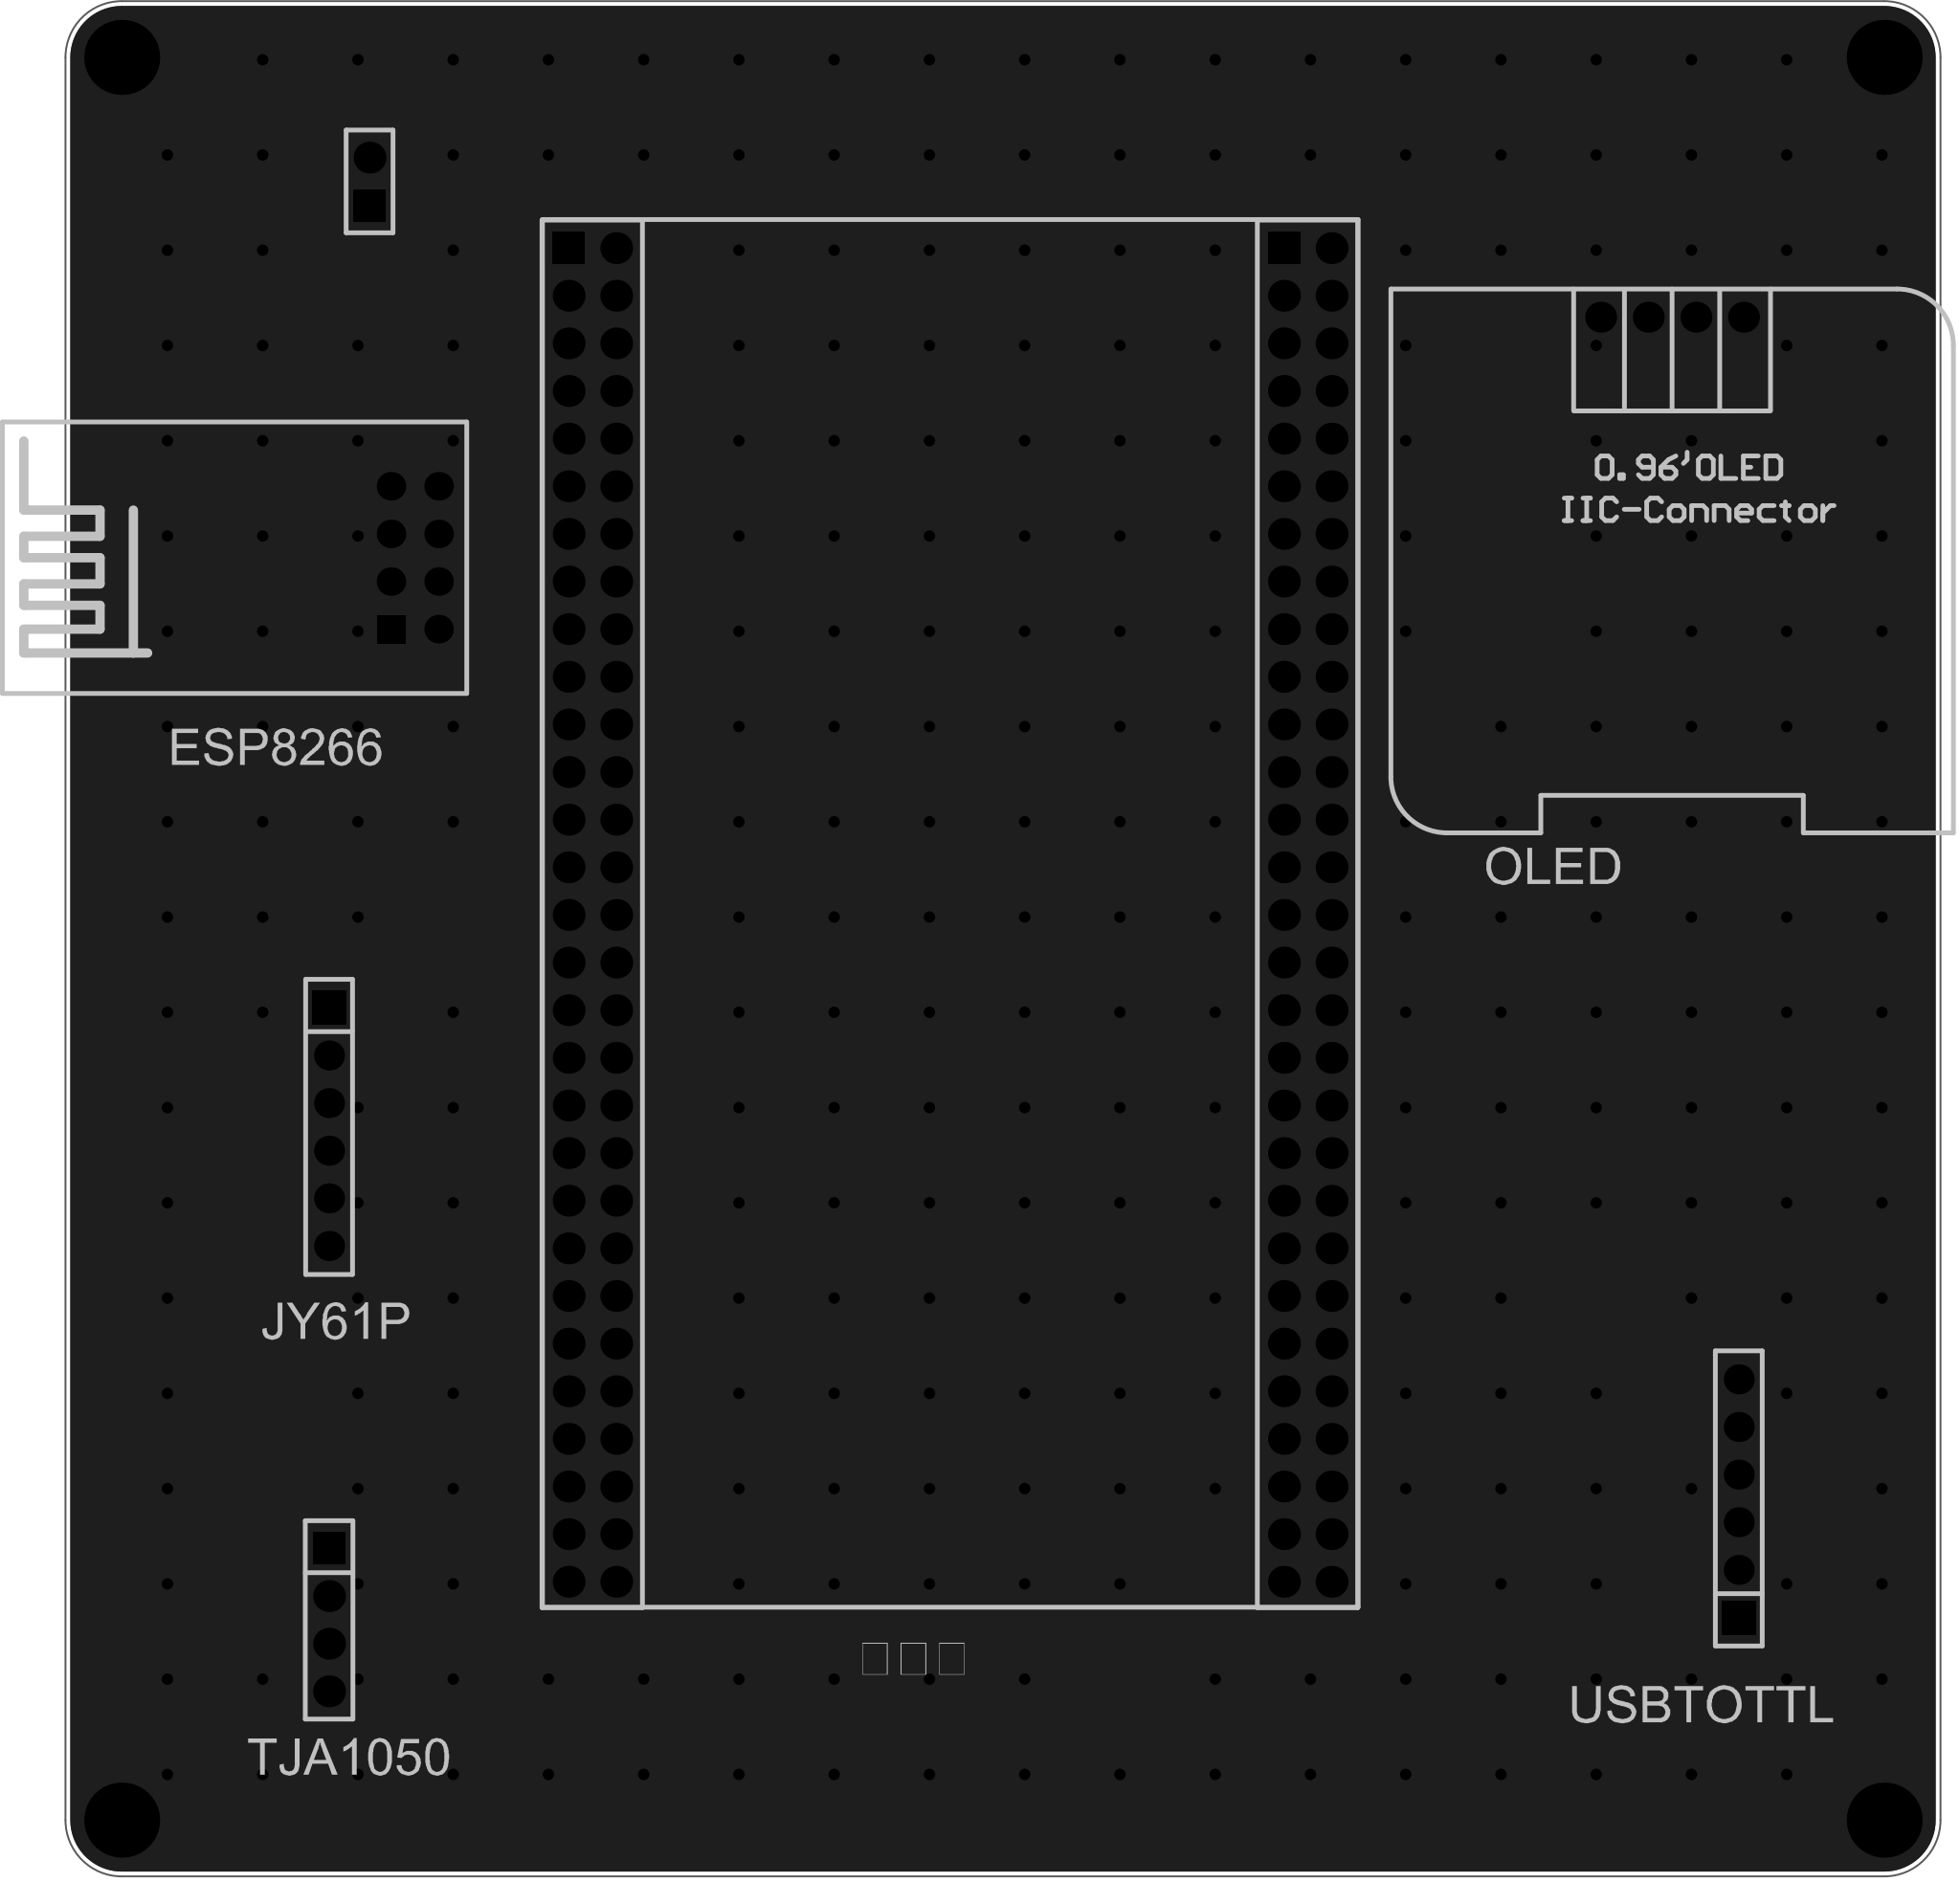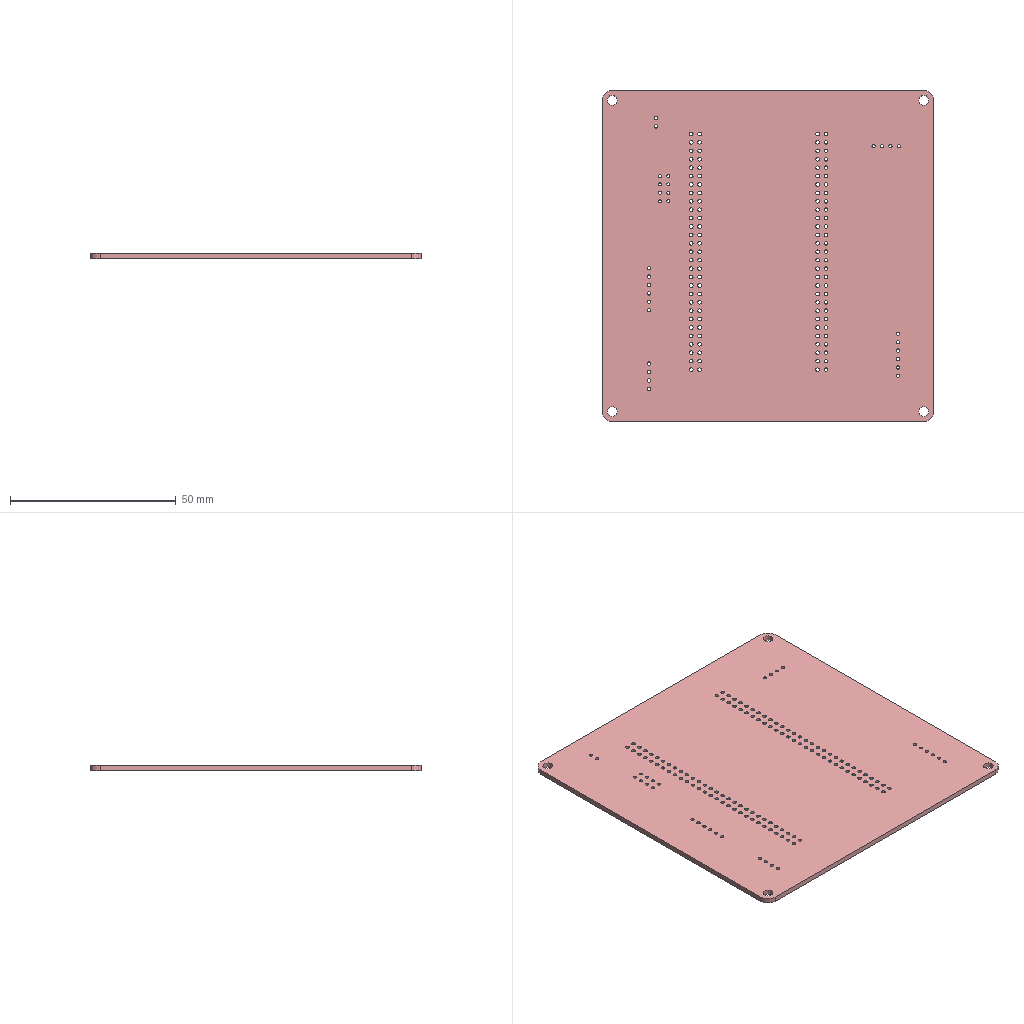Circuit board layout | Altium Designer | box 100 x 100 x 1.6 mm
Layer stack:
# Altium Designer layer stack of  (unit mm; dielectric type: 0 none, 1 core, 2 prepreg, 3 surface material)
index,name,kind,layer,copper_thickness_mm,dielectric_type,dielectric_thickness_mm,dielectric_material,dielectric_constant
0,Top Paste Mask Layer,other,,,,,,
1,Top Silkscreen Layer,other,,,,,,
2,Top Solder Mask Layer,dielectric,,,3,0.01,,3.3
3,Top Layer,copper,Top Layer,0.035,,,,
4,Dielectric1,dielectric,,,3,1.51,FR4,4.5
5,Bottom Layer,copper,Bottom Layer,0.035,,,,
6,Bottom Solder Mask Layer,dielectric,,,3,0.01,,3.3
7,Bottom Silkscreen Layer,other,,,,,,
8,Bottom Paste Mask Layer,other,,,,,,
# drill layer pairs: low layer,high layer
drill_pair,Top Layer,Bottom Layer
Part placement:
Designator,Comment,Layer,Footprint,Center-X(mm),Center-Y(mm),Rotation
H1,,TopLayer,HDR-TH_6P-P2.54-V-F,169.799,99.06,90
H8,,TopLayer,HDR-TH_4P-P2.54-V-F,94.615,92.583,270
H9,,TopLayer,HDR-TH_6P-P2.54-V-F,94.615,118.872,270
OLED1,,TopLayer,0.96OLED_4P,166.243,162.052,0
U1,XDFH-0254-2*30P,TopLayer,CONN-TH_60P-P2.54_LX_XDFH-0254-2X30P,146.812,130.175,270
U3,ESP8266-01S,TopLayer,WIFIM-TH_ESP8266-01S,99.187,149.225,90
U4,XDFH-0254-2*30P,TopLayer,CONN-TH_60P-P2.54_LX_XDFH-0254-2X30P,108.662,130.175,270
H2,,TopLayer,HDR-TH_2P-P2.54-V-F,96.774,169.291,90
Pad and via stacks:
# Altium Designer via and pad stacks of  (unit mm). Each distinct definition once, with the count of objects using it.
# via: kind,start_layer,end_layer,hole_mm,diameter_mm,mode(0 simple;1 top-mid-bottom;2 full stack),diameter_per_layer,count,example_net
# pad: kind,layer,hole_mm,hole_type(0 round;1 square;2 slot),plating,top_size,top_shape(1 round;2 rect;3 octagon;9 rounded rect),mid_size,bottom_size,mode,footprint,size_per_layer,count,example
pad,Multi-Layer,3,0,plated,4x4,1,4x4,4x4,0,,,4,1
pad,Multi-Layer,1.02,0,plated,1.6x1.6,1,1.6x1.6,1.6x1.6,0,HDR-TH_6P-P2.54-V-F,,10,H1.6
pad,Multi-Layer,1.02,0,plated,1.8x1.8,2,1.8x1.8,1.8x1.8,0,HDR-TH_6P-P2.54-V-F,,2,H1.1
pad,Multi-Layer,1.1,0,plated,1.7x1.7,2,1.7x1.7,1.7x1.7,0,HDR-TH_4P-P2.54-V-F,,1,H8.1
pad,Multi-Layer,1.1,0,plated,1.7x1.7,1,1.7x1.7,1.7x1.7,0,HDR-TH_4P-P2.54-V-F,,3,H8.2
pad,Multi-Layer,1,0,plated,1.65x1.65,1,1.65x1.65,1.65x1.65,0,0.96OLED_4P,,4,OLED1.4
pad,Multi-Layer,1.1,0,plated,1.7x1.7,2,1.7x1.7,1.7x1.7,0,CONN-TH_60P-P2.54_LX_XDFH-0254-2X30P,,2,U1.1
pad,Multi-Layer,1.1,0,plated,1.7x1.7,1,1.7x1.7,1.7x1.7,0,CONN-TH_60P-P2.54_LX_XDFH-0254-2X30P,,114,U1.2
pad,Multi-Layer,0.9144,0,plated,1.524x1.524,1,1.524x1.524,1.524x1.524,0,WIFIM-TH_ESP8266-01S,,7,U3.8
pad,Multi-Layer,0.9144,0,plated,1.524x1.524,2,1.524x1.524,1.524x1.524,0,WIFIM-TH_ESP8266-01S,,1,U3.1
pad,Multi-Layer,1,0,plated,1.7x1.7,2,1.7x1.7,1.7x1.7,0,HDR-TH_2P-P2.54-V-F,,1,H2.1
pad,Multi-Layer,1,0,plated,1.7x1.7,1,1.7x1.7,1.7x1.7,0,HDR-TH_2P-P2.54-V-F,,1,H2.2
via,Top Layer,Bottom Layer,0.3048,0.61,0,,288,GND
Copper pours:
name,layer,net,type(0 solid;1 hatched;2 none)
Bottom Layer-GND,Bottom Layer,GND,0
Top Layer-GND,Top Layer,GND,0
Design rules, without the lines most boards share:
# Altium Designer design rules of  (exported by Altium Designer, unit mm)
# columns: name | kind | enabled | priority | scope1 | scope2 | descriptor | typed fields (field=value)
copperThickness1oz_2 | 2 | enabled | 2 | All | All | Width Constraint (Min=5mil) (Max=100mil) (Preferred=30mil) (All) |
viaSize | 11 | enabled | 1 | All | All | Routing Via (MinHoleWidth=11.811mil) (MaxHoleWidth=248.032mil) (PreferredHoleWidth=12.008mil) (MinWidth=19.685mil) (MaxWidth=393.701mil) (PreferedWidth=24.016mil) (All) | via_min_hole=0.3 via_max_hole=6.3 via_preferred_diameter=0.61 via_preferred_hole=0.305
solderMaskExpansion | 13 | enabled | 2 | All | All | Solder Mask Expansion (Expansion =2.008mil) (All) | expansion=0.051